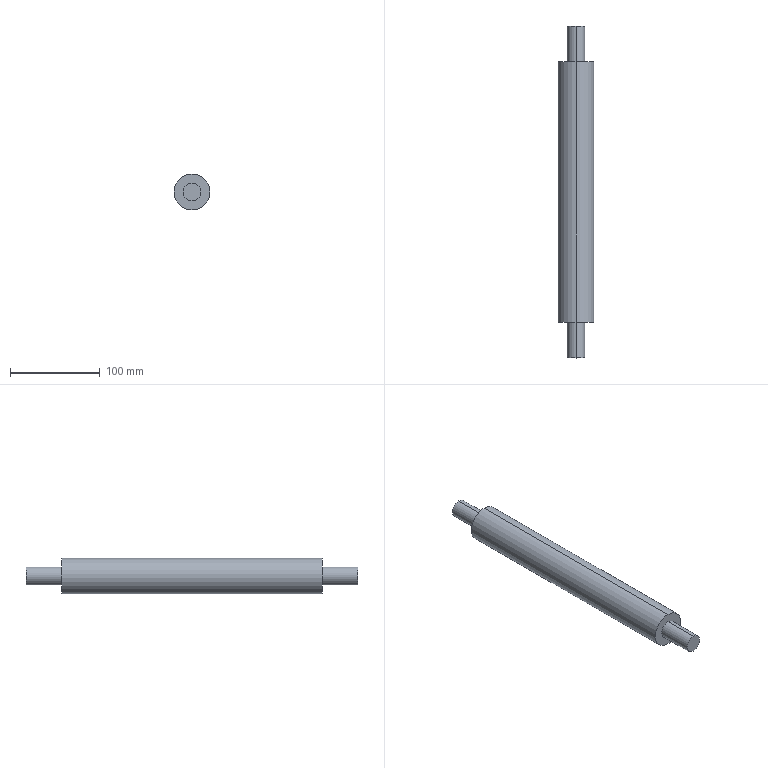Part | SolidWorks | features ICE 1, MirrorPattern 1, Revolution 1 | 1 solid | 20 faces | box 40 x 370 x 40 mm | volume 388983 mm3 | cylinder 10 | plane 10 | commonest cylinder face diameters 5 x4 20 x4 40 x2
STEP:
#1=CARTESIAN_POINT('',(0.,-145.,20.));
#2=VERTEX_POINT('',#1);
#3=CARTESIAN_POINT('',(0.,-145.,-20.));
#4=VERTEX_POINT('',#3);
#5=CARTESIAN_POINT('',(0.,-145.,0.));
#6=DIRECTION('',(0.,1.,0.));
#7=DIRECTION('',(0.,0.,1.));
#8=AXIS2_PLACEMENT_3D('',#5,#6,#7);
#9=CIRCLE('',#8,20.);
#10=EDGE_CURVE('',#2,#4,#9,.T.);
#11=ORIENTED_EDGE('',*,*,#10,.T.);
#12=CARTESIAN_POINT('',(0.,145.,-20.));
#13=VERTEX_POINT('',#12);
#14=CARTESIAN_POINT('',(0.,189.93,-20.));
#15=DIRECTION('',(0.,1.,0.));
#16=VECTOR('',#15,1000.);
#17=LINE('',#14,#16);
#18=EDGE_CURVE('',#4,#13,#17,.T.);
#19=ORIENTED_EDGE('',*,*,#18,.T.);
#20=CARTESIAN_POINT('',(0.,145.,20.));
#21=VERTEX_POINT('',#20);
#22=CARTESIAN_POINT('',(0.,145.,0.));
#23=DIRECTION('',(0.,1.,0.));
#24=DIRECTION('',(0.,0.,1.));
#25=AXIS2_PLACEMENT_3D('',#22,#23,#24);
#26=CIRCLE('',#25,20.);
#27=EDGE_CURVE('',#21,#13,#26,.T.);
#28=ORIENTED_EDGE('',*,*,#27,.F.);
#29=CARTESIAN_POINT('',(0.,189.93,20.));
#30=DIRECTION('',(0.,1.,0.));
#31=VECTOR('',#30,1000.);
#32=LINE('',#29,#31);
#33=EDGE_CURVE('',#2,#21,#32,.T.);
#34=ORIENTED_EDGE('',*,*,#33,.F.);
#35=EDGE_LOOP('',(#11,#19,#28,#34));
#36=FACE_OUTER_BOUND('',#35,.T.);
#37=CARTESIAN_POINT('',(0.,189.93,0.));
#38=DIRECTION('',(0.,1.,0.));
#39=DIRECTION('',(0.,0.,1.));
#40=AXIS2_PLACEMENT_3D('',#37,#38,#39);
#41=CYLINDRICAL_SURFACE('',#40,20.);
#42=ADVANCED_FACE('',(#36),#41,.T.);
#43=CARTESIAN_POINT('',(0.,145.,10.));
#44=VERTEX_POINT('',#43);
#45=CARTESIAN_POINT('',(0.,145.,-10.));
#46=VERTEX_POINT('',#45);
#47=CARTESIAN_POINT('',(0.,145.,0.));
#48=DIRECTION('',(0.,1.,0.));
#49=DIRECTION('',(0.,0.,1.));
#50=AXIS2_PLACEMENT_3D('',#47,#48,#49);
#51=CIRCLE('',#50,10.);
#52=EDGE_CURVE('',#44,#46,#51,.T.);
#53=ORIENTED_EDGE('',*,*,#52,.T.);
#54=CARTESIAN_POINT('',(0.,152.5,-10.));
#55=VERTEX_POINT('',#54);
#56=CARTESIAN_POINT('',(0.,189.93,-10.));
#57=DIRECTION('',(0.,1.,0.));
#58=VECTOR('',#57,1000.);
#59=LINE('',#56,#58);
#60=EDGE_CURVE('',#46,#55,#59,.T.);
#61=ORIENTED_EDGE('',*,*,#60,.T.);
#62=CARTESIAN_POINT('',(2.5,155.,-9.682));
#63=VERTEX_POINT('',#62);
#64=CARTESIAN_POINT('',(2.5,155.,-9.682));
#65=CARTESIAN_POINT('',(2.5,154.834,-9.682));
#66=CARTESIAN_POINT('',(2.484,154.671,-9.687));
#67=CARTESIAN_POINT('',(2.42,154.351,-9.703));
#68=CARTESIAN_POINT('',(2.371,154.191,-9.715));
#69=CARTESIAN_POINT('',(2.245,153.889,-9.745));
#70=CARTESIAN_POINT('',(2.169,153.745,-9.762));
#71=CARTESIAN_POINT('',(1.987,153.474,-9.801));
#72=CARTESIAN_POINT('',(1.882,153.346,-9.822));
#73=CARTESIAN_POINT('',(1.537,153.002,-9.884));
#74=CARTESIAN_POINT('',(1.259,152.816,-9.925));
#75=CARTESIAN_POINT('',(0.8081,152.629,-9.968));
#76=CARTESIAN_POINT('',(0.6497,152.58,-9.98));
#77=CARTESIAN_POINT('',(0.3266,152.516,-9.996));
#78=CARTESIAN_POINT('',(0.1638,152.5,-10.));
#79=CARTESIAN_POINT('',(0.,152.5,-10.));
#80=B_SPLINE_CURVE_WITH_KNOTS('',3,(#64,#65,#66,#67,#68,#69,#70,#71,#72,#73,#74,#75,#76,#77,#78,#79),.UNSPECIFIED.,.F.,.F.,(4,2,2,2,2,2,2,4),(0.,0.0004906,0.0009812,0.001472,0.001962,0.002944,0.003434,0.003925),.UNSPECIFIED.);
#81=EDGE_CURVE('',#63,#55,#80,.T.);
#82=ORIENTED_EDGE('',*,*,#81,.F.);
#83=CARTESIAN_POINT('',(2.5,175.,-9.682));
#84=VERTEX_POINT('',#83);
#85=CARTESIAN_POINT('',(2.5,189.93,-9.682));
#86=DIRECTION('',(0.,-1.,0.));
#87=VECTOR('',#86,1000.);
#88=LINE('',#85,#87);
#89=EDGE_CURVE('',#84,#63,#88,.T.);
#90=ORIENTED_EDGE('',*,*,#89,.F.);
#91=CARTESIAN_POINT('',(0.,177.5,-10.));
#92=VERTEX_POINT('',#91);
#93=CARTESIAN_POINT('',(0.,177.5,-10.));
#94=CARTESIAN_POINT('',(0.1637,177.5,-10.));
#95=CARTESIAN_POINT('',(0.3299,177.484,-9.996));
#96=CARTESIAN_POINT('',(0.6508,177.419,-9.98));
#97=CARTESIAN_POINT('',(0.8069,177.372,-9.969));
#98=CARTESIAN_POINT('',(1.262,177.183,-9.925));
#99=CARTESIAN_POINT('',(1.536,176.999,-9.884));
#100=CARTESIAN_POINT('',(1.884,176.652,-9.822));
#101=CARTESIAN_POINT('',(1.986,176.527,-9.801));
#102=CARTESIAN_POINT('',(2.167,176.257,-9.763));
#103=CARTESIAN_POINT('',(2.246,176.11,-9.745));
#104=CARTESIAN_POINT('',(2.371,175.809,-9.715));
#105=CARTESIAN_POINT('',(2.419,175.653,-9.703));
#106=CARTESIAN_POINT('',(2.483,175.332,-9.687));
#107=CARTESIAN_POINT('',(2.5,175.166,-9.682));
#108=CARTESIAN_POINT('',(2.5,175.,-9.682));
#109=B_SPLINE_CURVE_WITH_KNOTS('',3,(#93,#94,#95,#96,#97,#98,#99,#100,#101,#102,#103,#104,#105,#106,#107,#108),.UNSPECIFIED.,.F.,.F.,(4,2,2,2,2,2,2,4),(0.003925,0.004415,0.004905,0.005885,0.006375,0.006865,0.007355,0.007845),.UNSPECIFIED.);
#110=EDGE_CURVE('',#92,#84,#109,.T.);
#111=ORIENTED_EDGE('',*,*,#110,.F.);
#112=CARTESIAN_POINT('',(0.,185.,-10.));
#113=VERTEX_POINT('',#112);
#114=CARTESIAN_POINT('',(0.,189.93,-10.));
#115=DIRECTION('',(0.,1.,0.));
#116=VECTOR('',#115,1000.);
#117=LINE('',#114,#116);
#118=EDGE_CURVE('',#92,#113,#117,.T.);
#119=ORIENTED_EDGE('',*,*,#118,.T.);
#120=CARTESIAN_POINT('',(0.,185.,10.));
#121=VERTEX_POINT('',#120);
#122=CARTESIAN_POINT('',(0.,185.,0.));
#123=DIRECTION('',(0.,1.,0.));
#124=DIRECTION('',(0.,0.,1.));
#125=AXIS2_PLACEMENT_3D('',#122,#123,#124);
#126=CIRCLE('',#125,10.);
#127=EDGE_CURVE('',#121,#113,#126,.T.);
#128=ORIENTED_EDGE('',*,*,#127,.F.);
#129=CARTESIAN_POINT('',(0.,189.93,10.));
#130=DIRECTION('',(0.,1.,0.));
#131=VECTOR('',#130,1000.);
#132=LINE('',#129,#131);
#133=EDGE_CURVE('',#44,#121,#132,.T.);
#134=ORIENTED_EDGE('',*,*,#133,.F.);
#135=EDGE_LOOP('',(#53,#61,#82,#90,#111,#119,#128,#134));
#136=FACE_OUTER_BOUND('',#135,.T.);
#137=CARTESIAN_POINT('',(0.,189.93,0.));
#138=DIRECTION('',(0.,1.,0.));
#139=DIRECTION('',(0.,0.,1.));
#140=AXIS2_PLACEMENT_3D('',#137,#138,#139);
#141=CYLINDRICAL_SURFACE('',#140,10.);
#142=ADVANCED_FACE('',(#136),#141,.T.);
#143=CARTESIAN_POINT('',(0.,-185.,10.));
#144=VERTEX_POINT('',#143);
#145=CARTESIAN_POINT('',(0.,-185.,-10.));
#146=VERTEX_POINT('',#145);
#147=CARTESIAN_POINT('',(0.,-185.,0.));
#148=DIRECTION('',(0.,1.,0.));
#149=DIRECTION('',(0.,0.,1.));
#150=AXIS2_PLACEMENT_3D('',#147,#148,#149);
#151=CIRCLE('',#150,10.);
#152=EDGE_CURVE('',#144,#146,#151,.T.);
#153=ORIENTED_EDGE('',*,*,#152,.T.);
#154=CARTESIAN_POINT('',(0.,-177.5,-10.));
#155=VERTEX_POINT('',#154);
#156=CARTESIAN_POINT('',(0.,189.93,-10.));
#157=DIRECTION('',(0.,1.,0.));
#158=VECTOR('',#157,1000.);
#159=LINE('',#156,#158);
#160=EDGE_CURVE('',#146,#155,#159,.T.);
#161=ORIENTED_EDGE('',*,*,#160,.T.);
#162=CARTESIAN_POINT('',(2.5,-175.,-9.682));
#163=VERTEX_POINT('',#162);
#164=CARTESIAN_POINT('',(0.,-177.5,-10.));
#165=CARTESIAN_POINT('',(0.1637,-177.5,-10.));
#166=CARTESIAN_POINT('',(0.3299,-177.484,-9.996));
#167=CARTESIAN_POINT('',(0.6508,-177.419,-9.98));
#168=CARTESIAN_POINT('',(0.8069,-177.372,-9.969));
#169=CARTESIAN_POINT('',(1.262,-177.183,-9.925));
#170=CARTESIAN_POINT('',(1.536,-176.999,-9.884));
#171=CARTESIAN_POINT('',(1.884,-176.652,-9.822));
#172=CARTESIAN_POINT('',(1.986,-176.527,-9.801));
#173=CARTESIAN_POINT('',(2.167,-176.257,-9.763));
#174=CARTESIAN_POINT('',(2.246,-176.11,-9.745));
#175=CARTESIAN_POINT('',(2.371,-175.809,-9.715));
#176=CARTESIAN_POINT('',(2.419,-175.653,-9.703));
#177=CARTESIAN_POINT('',(2.483,-175.332,-9.687));
#178=CARTESIAN_POINT('',(2.5,-175.166,-9.682));
#179=CARTESIAN_POINT('',(2.5,-175.,-9.682));
#180=B_SPLINE_CURVE_WITH_KNOTS('',3,(#164,#165,#166,#167,#168,#169,#170,#171,#172,#173,#174,#175,#176,#177,#178,#179),.UNSPECIFIED.,.F.,.F.,(4,2,2,2,2,2,2,4),(0.003925,0.004415,0.004905,0.005885,0.006375,0.006865,0.007355,0.007845),.UNSPECIFIED.);
#181=EDGE_CURVE('',#155,#163,#180,.T.);
#182=ORIENTED_EDGE('',*,*,#181,.T.);
#183=CARTESIAN_POINT('',(2.5,-155.,-9.682));
#184=VERTEX_POINT('',#183);
#185=CARTESIAN_POINT('',(2.5,189.93,-9.682));
#186=DIRECTION('',(0.,1.,0.));
#187=VECTOR('',#186,1000.);
#188=LINE('',#185,#187);
#189=EDGE_CURVE('',#163,#184,#188,.T.);
#190=ORIENTED_EDGE('',*,*,#189,.T.);
#191=CARTESIAN_POINT('',(0.,-152.5,-10.));
#192=VERTEX_POINT('',#191);
#193=CARTESIAN_POINT('',(2.5,-155.,-9.682));
#194=CARTESIAN_POINT('',(2.5,-154.834,-9.682));
#195=CARTESIAN_POINT('',(2.484,-154.671,-9.687));
#196=CARTESIAN_POINT('',(2.42,-154.351,-9.703));
#197=CARTESIAN_POINT('',(2.371,-154.191,-9.715));
#198=CARTESIAN_POINT('',(2.245,-153.889,-9.745));
#199=CARTESIAN_POINT('',(2.169,-153.745,-9.762));
#200=CARTESIAN_POINT('',(1.987,-153.474,-9.801));
#201=CARTESIAN_POINT('',(1.882,-153.346,-9.822));
#202=CARTESIAN_POINT('',(1.537,-153.002,-9.884));
#203=CARTESIAN_POINT('',(1.259,-152.816,-9.925));
#204=CARTESIAN_POINT('',(0.8081,-152.629,-9.968));
#205=CARTESIAN_POINT('',(0.6497,-152.58,-9.98));
#206=CARTESIAN_POINT('',(0.3266,-152.516,-9.996));
#207=CARTESIAN_POINT('',(0.1638,-152.5,-10.));
#208=CARTESIAN_POINT('',(0.,-152.5,-10.));
#209=B_SPLINE_CURVE_WITH_KNOTS('',3,(#193,#194,#195,#196,#197,#198,#199,#200,#201,#202,#203,#204,#205,#206,#207,#208),.UNSPECIFIED.,.F.,.F.,(4,2,2,2,2,2,2,4),(0.,0.0004906,0.0009812,0.001472,0.001962,0.002944,0.003434,0.003925),.UNSPECIFIED.);
#210=EDGE_CURVE('',#184,#192,#209,.T.);
#211=ORIENTED_EDGE('',*,*,#210,.T.);
#212=CARTESIAN_POINT('',(0.,-145.,-10.));
#213=VERTEX_POINT('',#212);
#214=CARTESIAN_POINT('',(0.,189.93,-10.));
#215=DIRECTION('',(0.,1.,0.));
#216=VECTOR('',#215,1000.);
#217=LINE('',#214,#216);
#218=EDGE_CURVE('',#192,#213,#217,.T.);
#219=ORIENTED_EDGE('',*,*,#218,.T.);
#220=CARTESIAN_POINT('',(0.,-145.,10.));
#221=VERTEX_POINT('',#220);
#222=CARTESIAN_POINT('',(0.,-145.,0.));
#223=DIRECTION('',(0.,1.,0.));
#224=DIRECTION('',(0.,0.,1.));
#225=AXIS2_PLACEMENT_3D('',#222,#223,#224);
#226=CIRCLE('',#225,10.);
#227=EDGE_CURVE('',#221,#213,#226,.T.);
#228=ORIENTED_EDGE('',*,*,#227,.F.);
#229=CARTESIAN_POINT('',(0.,189.93,10.));
#230=DIRECTION('',(0.,1.,0.));
#231=VECTOR('',#230,1000.);
#232=LINE('',#229,#231);
#233=EDGE_CURVE('',#144,#221,#232,.T.);
#234=ORIENTED_EDGE('',*,*,#233,.F.);
#235=EDGE_LOOP('',(#153,#161,#182,#190,#211,#219,#228,#234));
#236=FACE_OUTER_BOUND('',#235,.T.);
#237=CARTESIAN_POINT('',(0.,189.93,0.));
#238=DIRECTION('',(0.,1.,0.));
#239=DIRECTION('',(0.,0.,1.));
#240=AXIS2_PLACEMENT_3D('',#237,#238,#239);
#241=CYLINDRICAL_SURFACE('',#240,10.);
#242=ADVANCED_FACE('',(#236),#241,.T.);
#243=ORIENTED_EDGE('',*,*,#160,.F.);
#244=CARTESIAN_POINT('',(0.,-185.,0.));
#245=DIRECTION('',(0.,1.,0.));
#246=DIRECTION('',(0.,0.,1.));
#247=AXIS2_PLACEMENT_3D('',#244,#245,#246);
#248=CIRCLE('',#247,10.);
#249=EDGE_CURVE('',#146,#144,#248,.T.);
#250=ORIENTED_EDGE('',*,*,#249,.T.);
#251=ORIENTED_EDGE('',*,*,#233,.T.);
#252=CARTESIAN_POINT('',(0.,-145.,0.));
#253=DIRECTION('',(0.,1.,0.));
#254=DIRECTION('',(0.,0.,1.));
#255=AXIS2_PLACEMENT_3D('',#252,#253,#254);
#256=CIRCLE('',#255,10.);
#257=EDGE_CURVE('',#213,#221,#256,.T.);
#258=ORIENTED_EDGE('',*,*,#257,.F.);
#259=ORIENTED_EDGE('',*,*,#218,.F.);
#260=CARTESIAN_POINT('',(-2.5,-155.,-9.682));
#261=VERTEX_POINT('',#260);
#262=CARTESIAN_POINT('',(0.,-152.5,-10.));
#263=CARTESIAN_POINT('',(-0.1637,-152.5,-10.));
#264=CARTESIAN_POINT('',(-0.3299,-152.516,-9.996));
#265=CARTESIAN_POINT('',(-0.6508,-152.581,-9.98));
#266=CARTESIAN_POINT('',(-0.8069,-152.628,-9.969));
#267=CARTESIAN_POINT('',(-1.262,-152.817,-9.925));
#268=CARTESIAN_POINT('',(-1.536,-153.001,-9.884));
#269=CARTESIAN_POINT('',(-1.884,-153.348,-9.822));
#270=CARTESIAN_POINT('',(-1.986,-153.473,-9.801));
#271=CARTESIAN_POINT('',(-2.167,-153.743,-9.763));
#272=CARTESIAN_POINT('',(-2.246,-153.89,-9.745));
#273=CARTESIAN_POINT('',(-2.371,-154.191,-9.715));
#274=CARTESIAN_POINT('',(-2.419,-154.347,-9.703));
#275=CARTESIAN_POINT('',(-2.483,-154.668,-9.687));
#276=CARTESIAN_POINT('',(-2.5,-154.834,-9.682));
#277=CARTESIAN_POINT('',(-2.5,-155.,-9.682));
#278=B_SPLINE_CURVE_WITH_KNOTS('',3,(#262,#263,#264,#265,#266,#267,#268,#269,#270,#271,#272,#273,#274,#275,#276,#277),.UNSPECIFIED.,.F.,.F.,(4,2,2,2,2,2,2,4),(0.003925,0.004415,0.004905,0.005885,0.006375,0.006865,0.007355,0.007845),.UNSPECIFIED.);
#279=EDGE_CURVE('',#192,#261,#278,.T.);
#280=ORIENTED_EDGE('',*,*,#279,.T.);
#281=CARTESIAN_POINT('',(-2.5,-175.,-9.682));
#282=VERTEX_POINT('',#281);
#283=CARTESIAN_POINT('',(-2.5,189.93,-9.682));
#284=DIRECTION('',(0.,-1.,0.));
#285=VECTOR('',#284,1000.);
#286=LINE('',#283,#285);
#287=EDGE_CURVE('',#261,#282,#286,.T.);
#288=ORIENTED_EDGE('',*,*,#287,.T.);
#289=CARTESIAN_POINT('',(-2.5,-175.,-9.682));
#290=CARTESIAN_POINT('',(-2.5,-175.166,-9.682));
#291=CARTESIAN_POINT('',(-2.484,-175.329,-9.687));
#292=CARTESIAN_POINT('',(-2.42,-175.649,-9.703));
#293=CARTESIAN_POINT('',(-2.371,-175.809,-9.715));
#294=CARTESIAN_POINT('',(-2.245,-176.111,-9.745));
#295=CARTESIAN_POINT('',(-2.169,-176.255,-9.762));
#296=CARTESIAN_POINT('',(-1.987,-176.526,-9.801));
#297=CARTESIAN_POINT('',(-1.882,-176.654,-9.822));
#298=CARTESIAN_POINT('',(-1.537,-176.998,-9.884));
#299=CARTESIAN_POINT('',(-1.259,-177.184,-9.925));
#300=CARTESIAN_POINT('',(-0.8081,-177.371,-9.968));
#301=CARTESIAN_POINT('',(-0.6497,-177.42,-9.98));
#302=CARTESIAN_POINT('',(-0.3266,-177.484,-9.996));
#303=CARTESIAN_POINT('',(-0.1638,-177.5,-10.));
#304=CARTESIAN_POINT('',(0.,-177.5,-10.));
#305=B_SPLINE_CURVE_WITH_KNOTS('',3,(#289,#290,#291,#292,#293,#294,#295,#296,#297,#298,#299,#300,#301,#302,#303,#304),.UNSPECIFIED.,.F.,.F.,(4,2,2,2,2,2,2,4),(0.,0.0004906,0.0009812,0.001472,0.001962,0.002944,0.003434,0.003925),.UNSPECIFIED.);
#306=EDGE_CURVE('',#282,#155,#305,.T.);
#307=ORIENTED_EDGE('',*,*,#306,.T.);
#308=EDGE_LOOP('',(#243,#250,#251,#258,#259,#280,#288,#307));
#309=FACE_OUTER_BOUND('',#308,.T.);
#310=CARTESIAN_POINT('',(0.,189.93,0.));
#311=DIRECTION('',(0.,1.,0.));
#312=DIRECTION('',(0.,0.,1.));
#313=AXIS2_PLACEMENT_3D('',#310,#311,#312);
#314=CYLINDRICAL_SURFACE('',#313,10.);
#315=ADVANCED_FACE('',(#309),#314,.T.);
#316=ORIENTED_EDGE('',*,*,#127,.T.);
#317=CARTESIAN_POINT('',(0.,185.,0.));
#318=DIRECTION('',(0.,1.,0.));
#319=DIRECTION('',(0.,0.,1.));
#320=AXIS2_PLACEMENT_3D('',#317,#318,#319);
#321=CIRCLE('',#320,10.);
#322=EDGE_CURVE('',#113,#121,#321,.T.);
#323=ORIENTED_EDGE('',*,*,#322,.T.);
#324=EDGE_LOOP('',(#316,#323));
#325=FACE_OUTER_BOUND('',#324,.T.);
#326=CARTESIAN_POINT('',(0.,185.,0.));
#327=DIRECTION('',(0.,1.,0.));
#328=DIRECTION('',(0.,0.,1.));
#329=AXIS2_PLACEMENT_3D('',#326,#327,#328);
#330=PLANE('',#329);
#331=ADVANCED_FACE('',(#325),#330,.T.);
#332=ORIENTED_EDGE('',*,*,#60,.F.);
#333=CARTESIAN_POINT('',(0.,145.,0.));
#334=DIRECTION('',(0.,1.,0.));
#335=DIRECTION('',(0.,0.,1.));
#336=AXIS2_PLACEMENT_3D('',#333,#334,#335);
#337=CIRCLE('',#336,10.);
#338=EDGE_CURVE('',#46,#44,#337,.T.);
#339=ORIENTED_EDGE('',*,*,#338,.T.);
#340=ORIENTED_EDGE('',*,*,#133,.T.);
#341=ORIENTED_EDGE('',*,*,#322,.F.);
#342=ORIENTED_EDGE('',*,*,#118,.F.);
#343=CARTESIAN_POINT('',(-2.5,175.,-9.682));
#344=VERTEX_POINT('',#343);
#345=CARTESIAN_POINT('',(-2.5,175.,-9.682));
#346=CARTESIAN_POINT('',(-2.5,175.166,-9.682));
#347=CARTESIAN_POINT('',(-2.484,175.329,-9.687));
#348=CARTESIAN_POINT('',(-2.42,175.649,-9.703));
#349=CARTESIAN_POINT('',(-2.371,175.809,-9.715));
#350=CARTESIAN_POINT('',(-2.245,176.111,-9.745));
#351=CARTESIAN_POINT('',(-2.169,176.255,-9.762));
#352=CARTESIAN_POINT('',(-1.987,176.526,-9.801));
#353=CARTESIAN_POINT('',(-1.882,176.654,-9.822));
#354=CARTESIAN_POINT('',(-1.537,176.998,-9.884));
#355=CARTESIAN_POINT('',(-1.259,177.184,-9.925));
#356=CARTESIAN_POINT('',(-0.8081,177.371,-9.968));
#357=CARTESIAN_POINT('',(-0.6497,177.42,-9.98));
#358=CARTESIAN_POINT('',(-0.3266,177.484,-9.996));
#359=CARTESIAN_POINT('',(-0.1638,177.5,-10.));
#360=CARTESIAN_POINT('',(0.,177.5,-10.));
#361=B_SPLINE_CURVE_WITH_KNOTS('',3,(#345,#346,#347,#348,#349,#350,#351,#352,#353,#354,#355,#356,#357,#358,#359,#360),.UNSPECIFIED.,.F.,.F.,(4,2,2,2,2,2,2,4),(0.,0.0004906,0.0009812,0.001472,0.001962,0.002944,0.003434,0.003925),.UNSPECIFIED.);
#362=EDGE_CURVE('',#344,#92,#361,.T.);
#363=ORIENTED_EDGE('',*,*,#362,.F.);
#364=CARTESIAN_POINT('',(-2.5,155.,-9.682));
#365=VERTEX_POINT('',#364);
#366=CARTESIAN_POINT('',(-2.5,189.93,-9.682));
#367=DIRECTION('',(0.,1.,0.));
#368=VECTOR('',#367,1000.);
#369=LINE('',#366,#368);
#370=EDGE_CURVE('',#365,#344,#369,.T.);
#371=ORIENTED_EDGE('',*,*,#370,.F.);
#372=CARTESIAN_POINT('',(0.,152.5,-10.));
#373=CARTESIAN_POINT('',(-0.1637,152.5,-10.));
#374=CARTESIAN_POINT('',(-0.3299,152.516,-9.996));
#375=CARTESIAN_POINT('',(-0.6508,152.581,-9.98));
#376=CARTESIAN_POINT('',(-0.8069,152.628,-9.969));
#377=CARTESIAN_POINT('',(-1.262,152.817,-9.925));
#378=CARTESIAN_POINT('',(-1.536,153.001,-9.884));
#379=CARTESIAN_POINT('',(-1.884,153.348,-9.822));
#380=CARTESIAN_POINT('',(-1.986,153.473,-9.801));
#381=CARTESIAN_POINT('',(-2.167,153.743,-9.763));
#382=CARTESIAN_POINT('',(-2.246,153.89,-9.745));
#383=CARTESIAN_POINT('',(-2.371,154.191,-9.715));
#384=CARTESIAN_POINT('',(-2.419,154.347,-9.703));
#385=CARTESIAN_POINT('',(-2.483,154.668,-9.687));
#386=CARTESIAN_POINT('',(-2.5,154.834,-9.682));
#387=CARTESIAN_POINT('',(-2.5,155.,-9.682));
#388=B_SPLINE_CURVE_WITH_KNOTS('',3,(#372,#373,#374,#375,#376,#377,#378,#379,#380,#381,#382,#383,#384,#385,#386,#387),.UNSPECIFIED.,.F.,.F.,(4,2,2,2,2,2,2,4),(0.003925,0.004415,0.004905,0.005885,0.006375,0.006865,0.007355,0.007845),.UNSPECIFIED.);
#389=EDGE_CURVE('',#55,#365,#388,.T.);
#390=ORIENTED_EDGE('',*,*,#389,.F.);
#391=EDGE_LOOP('',(#332,#339,#340,#341,#342,#363,#371,#390));
#392=FACE_OUTER_BOUND('',#391,.T.);
#393=CARTESIAN_POINT('',(0.,189.93,0.));
#394=DIRECTION('',(0.,1.,0.));
#395=DIRECTION('',(0.,0.,1.));
#396=AXIS2_PLACEMENT_3D('',#393,#394,#395);
#397=CYLINDRICAL_SURFACE('',#396,10.);
#398=ADVANCED_FACE('',(#392),#397,.T.);
#399=ORIENTED_EDGE('',*,*,#27,.T.);
#400=CARTESIAN_POINT('',(0.,145.,0.));
#401=DIRECTION('',(0.,1.,0.));
#402=DIRECTION('',(0.,0.,1.));
#403=AXIS2_PLACEMENT_3D('',#400,#401,#402);
#404=CIRCLE('',#403,20.);
#405=EDGE_CURVE('',#13,#21,#404,.T.);
#406=ORIENTED_EDGE('',*,*,#405,.T.);
#407=EDGE_LOOP('',(#399,#406));
#408=FACE_OUTER_BOUND('',#407,.T.);
#409=ORIENTED_EDGE('',*,*,#52,.F.);
#410=ORIENTED_EDGE('',*,*,#338,.F.);
#411=EDGE_LOOP('',(#409,#410));
#412=FACE_BOUND('',#411,.T.);
#413=CARTESIAN_POINT('',(0.,145.,10.));
#414=DIRECTION('',(0.,1.,0.));
#415=DIRECTION('',(0.,0.,1.));
#416=AXIS2_PLACEMENT_3D('',#413,#414,#415);
#417=PLANE('',#416);
#418=ADVANCED_FACE('',(#408,#412),#417,.T.);
#419=ORIENTED_EDGE('',*,*,#18,.F.);
#420=CARTESIAN_POINT('',(0.,-145.,0.));
#421=DIRECTION('',(0.,1.,0.));
#422=DIRECTION('',(0.,0.,1.));
#423=AXIS2_PLACEMENT_3D('',#420,#421,#422);
#424=CIRCLE('',#423,20.);
#425=EDGE_CURVE('',#4,#2,#424,.T.);
#426=ORIENTED_EDGE('',*,*,#425,.T.);
#427=ORIENTED_EDGE('',*,*,#33,.T.);
#428=ORIENTED_EDGE('',*,*,#405,.F.);
#429=EDGE_LOOP('',(#419,#426,#427,#428));
#430=FACE_OUTER_BOUND('',#429,.T.);
#431=CARTESIAN_POINT('',(0.,189.93,0.));
#432=DIRECTION('',(0.,1.,0.));
#433=DIRECTION('',(0.,0.,1.));
#434=AXIS2_PLACEMENT_3D('',#431,#432,#433);
#435=CYLINDRICAL_SURFACE('',#434,20.);
#436=ADVANCED_FACE('',(#430),#435,.T.);
#437=ORIENTED_EDGE('',*,*,#227,.T.);
#438=ORIENTED_EDGE('',*,*,#257,.T.);
#439=EDGE_LOOP('',(#437,#438));
#440=FACE_BOUND('',#439,.T.);
#441=ORIENTED_EDGE('',*,*,#10,.F.);
#442=ORIENTED_EDGE('',*,*,#425,.F.);
#443=EDGE_LOOP('',(#441,#442));
#444=FACE_OUTER_BOUND('',#443,.T.);
#445=CARTESIAN_POINT('',(0.,-145.,20.));
#446=DIRECTION('',(0.,-1.,0.));
#447=DIRECTION('',(0.,0.,-1.));
#448=AXIS2_PLACEMENT_3D('',#445,#446,#447);
#449=PLANE('',#448);
#450=ADVANCED_FACE('',(#440,#444),#449,.T.);
#451=ORIENTED_EDGE('',*,*,#152,.F.);
#452=ORIENTED_EDGE('',*,*,#249,.F.);
#453=EDGE_LOOP('',(#451,#452));
#454=FACE_OUTER_BOUND('',#453,.T.);
#455=CARTESIAN_POINT('',(0.,-185.,10.));
#456=DIRECTION('',(0.,-1.,0.));
#457=DIRECTION('',(0.,0.,-1.));
#458=AXIS2_PLACEMENT_3D('',#455,#456,#457);
#459=PLANE('',#458);
#460=ADVANCED_FACE('',(#454),#459,.T.);
#461=CARTESIAN_POINT('',(-2.5,175.,-7.5));
#462=VERTEX_POINT('',#461);
#463=CARTESIAN_POINT('',(-2.5,175.,-7.5));
#464=DIRECTION('',(0.,0.,-1.));
#465=VECTOR('',#464,1000.);
#466=LINE('',#463,#465);
#467=EDGE_CURVE('',#462,#344,#466,.T.);
#468=ORIENTED_EDGE('',*,*,#467,.T.);
#469=ORIENTED_EDGE('',*,*,#362,.T.);
#470=ORIENTED_EDGE('',*,*,#110,.T.);
#471=CARTESIAN_POINT('',(2.5,175.,-7.5));
#472=VERTEX_POINT('',#471);
#473=CARTESIAN_POINT('',(2.5,175.,-7.5));
#474=DIRECTION('',(0.,0.,-1.));
#475=VECTOR('',#474,1000.);
#476=LINE('',#473,#475);
#477=EDGE_CURVE('',#472,#84,#476,.T.);
#478=ORIENTED_EDGE('',*,*,#477,.F.);
#479=CARTESIAN_POINT('',(0.,175.,-7.5));
#480=DIRECTION('',(0.,0.,-1.));
#481=DIRECTION('',(-1.,0.,0.));
#482=AXIS2_PLACEMENT_3D('',#479,#480,#481);
#483=CIRCLE('',#482,2.5);
#484=EDGE_CURVE('',#462,#472,#483,.T.);
#485=ORIENTED_EDGE('',*,*,#484,.F.);
#486=EDGE_LOOP('',(#468,#469,#470,#478,#485));
#487=FACE_OUTER_BOUND('',#486,.T.);
#488=CARTESIAN_POINT('',(0.,175.,-7.5));
#489=DIRECTION('',(0.,0.,-1.));
#490=DIRECTION('',(-1.,0.,0.));
#491=AXIS2_PLACEMENT_3D('',#488,#489,#490);
#492=CYLINDRICAL_SURFACE('',#491,2.5);
#493=ADVANCED_FACE('',(#487),#492,.F.);
#494=ORIENTED_EDGE('',*,*,#370,.T.);
#495=ORIENTED_EDGE('',*,*,#467,.F.);
#496=CARTESIAN_POINT('',(-2.5,155.,-7.5));
#497=VERTEX_POINT('',#496);
#498=CARTESIAN_POINT('',(-2.5,175.,-7.5));
#499=DIRECTION('',(0.,1.,0.));
#500=VECTOR('',#499,1000.);
#501=LINE('',#498,#500);
#502=EDGE_CURVE('',#497,#462,#501,.T.);
#503=ORIENTED_EDGE('',*,*,#502,.F.);
#504=CARTESIAN_POINT('',(-2.5,155.,-7.5));
#505=DIRECTION('',(0.,0.,-1.));
#506=VECTOR('',#505,1000.);
#507=LINE('',#504,#506);
#508=EDGE_CURVE('',#497,#365,#507,.T.);
#509=ORIENTED_EDGE('',*,*,#508,.T.);
#510=EDGE_LOOP('',(#494,#495,#503,#509));
#511=FACE_OUTER_BOUND('',#510,.T.);
#512=CARTESIAN_POINT('',(-2.5,175.,-7.5));
#513=DIRECTION('',(-1.,0.,0.));
#514=DIRECTION('',(0.,-1.,0.));
#515=AXIS2_PLACEMENT_3D('',#512,#513,#514);
#516=PLANE('',#515);
#517=ADVANCED_FACE('',(#511),#516,.F.);
#518=CARTESIAN_POINT('',(2.5,155.,-7.5));
#519=VERTEX_POINT('',#518);
#520=CARTESIAN_POINT('',(2.5,155.,-7.5));
#521=DIRECTION('',(0.,0.,-1.));
#522=VECTOR('',#521,1000.);
#523=LINE('',#520,#522);
#524=EDGE_CURVE('',#519,#63,#523,.T.);
#525=ORIENTED_EDGE('',*,*,#524,.T.);
#526=ORIENTED_EDGE('',*,*,#81,.T.);
#527=ORIENTED_EDGE('',*,*,#389,.T.);
#528=ORIENTED_EDGE('',*,*,#508,.F.);
#529=CARTESIAN_POINT('',(0.,155.,-7.5));
#530=DIRECTION('',(0.,0.,-1.));
#531=DIRECTION('',(-1.,0.,0.));
#532=AXIS2_PLACEMENT_3D('',#529,#530,#531);
#533=CIRCLE('',#532,2.5);
#534=EDGE_CURVE('',#519,#497,#533,.T.);
#535=ORIENTED_EDGE('',*,*,#534,.F.);
#536=EDGE_LOOP('',(#525,#526,#527,#528,#535));
#537=FACE_OUTER_BOUND('',#536,.T.);
#538=CARTESIAN_POINT('',(0.,155.,-7.5));
#539=DIRECTION('',(0.,0.,-1.));
#540=DIRECTION('',(-1.,0.,0.));
#541=AXIS2_PLACEMENT_3D('',#538,#539,#540);
#542=CYLINDRICAL_SURFACE('',#541,2.5);
#543=ADVANCED_FACE('',(#537),#542,.F.);
#544=ORIENTED_EDGE('',*,*,#89,.T.);
#545=ORIENTED_EDGE('',*,*,#524,.F.);
#546=CARTESIAN_POINT('',(2.5,175.,-7.5));
#547=DIRECTION('',(0.,-1.,0.));
#548=VECTOR('',#547,1000.);
#549=LINE('',#546,#548);
#550=EDGE_CURVE('',#472,#519,#549,.T.);
#551=ORIENTED_EDGE('',*,*,#550,.F.);
#552=ORIENTED_EDGE('',*,*,#477,.T.);
#553=EDGE_LOOP('',(#544,#545,#551,#552));
#554=FACE_OUTER_BOUND('',#553,.T.);
#555=CARTESIAN_POINT('',(2.5,175.,-7.5));
#556=DIRECTION('',(1.,0.,0.));
#557=DIRECTION('',(0.,1.,0.));
#558=AXIS2_PLACEMENT_3D('',#555,#556,#557);
#559=PLANE('',#558);
#560=ADVANCED_FACE('',(#554),#559,.F.);
#561=ORIENTED_EDGE('',*,*,#484,.T.);
#562=ORIENTED_EDGE('',*,*,#550,.T.);
#563=ORIENTED_EDGE('',*,*,#534,.T.);
#564=ORIENTED_EDGE('',*,*,#502,.T.);
#565=EDGE_LOOP('',(#561,#562,#563,#564));
#566=FACE_OUTER_BOUND('',#565,.T.);
#567=CARTESIAN_POINT('',(0.,175.,-7.5));
#568=DIRECTION('',(0.,0.,-1.));
#569=DIRECTION('',(-1.,0.,0.));
#570=AXIS2_PLACEMENT_3D('',#567,#568,#569);
#571=PLANE('',#570);
#572=ADVANCED_FACE('',(#566),#571,.T.);
#573=CARTESIAN_POINT('',(-2.5,-175.,-7.5));
#574=VERTEX_POINT('',#573);
#575=CARTESIAN_POINT('',(-2.5,-175.,-7.5));
#576=DIRECTION('',(0.,0.,-1.));
#577=VECTOR('',#576,1000.);
#578=LINE('',#575,#577);
#579=EDGE_CURVE('',#574,#282,#578,.T.);
#580=ORIENTED_EDGE('',*,*,#579,.F.);
#581=CARTESIAN_POINT('',(2.5,-175.,-7.5));
#582=VERTEX_POINT('',#581);
#583=CARTESIAN_POINT('',(0.,-175.,-7.5));
#584=DIRECTION('',(0.,0.,1.));
#585=DIRECTION('',(-1.,0.,0.));
#586=AXIS2_PLACEMENT_3D('',#583,#584,#585);
#587=CIRCLE('',#586,2.5);
#588=EDGE_CURVE('',#574,#582,#587,.T.);
#589=ORIENTED_EDGE('',*,*,#588,.T.);
#590=CARTESIAN_POINT('',(2.5,-175.,-7.5));
#591=DIRECTION('',(0.,0.,-1.));
#592=VECTOR('',#591,1000.);
#593=LINE('',#590,#592);
#594=EDGE_CURVE('',#582,#163,#593,.T.);
#595=ORIENTED_EDGE('',*,*,#594,.T.);
#596=ORIENTED_EDGE('',*,*,#181,.F.);
#597=ORIENTED_EDGE('',*,*,#306,.F.);
#598=EDGE_LOOP('',(#580,#589,#595,#596,#597));
#599=FACE_OUTER_BOUND('',#598,.T.);
#600=CARTESIAN_POINT('',(0.,-175.,-7.5));
#601=DIRECTION('',(0.,0.,-1.));
#602=DIRECTION('',(-1.,0.,0.));
#603=AXIS2_PLACEMENT_3D('',#600,#601,#602);
#604=CYLINDRICAL_SURFACE('',#603,2.5);
#605=ADVANCED_FACE('',(#599),#604,.F.);
#606=ORIENTED_EDGE('',*,*,#594,.F.);
#607=CARTESIAN_POINT('',(2.5,-155.,-7.5));
#608=VERTEX_POINT('',#607);
#609=CARTESIAN_POINT('',(2.5,-175.,-7.5));
#610=DIRECTION('',(0.,1.,0.));
#611=VECTOR('',#610,1000.);
#612=LINE('',#609,#611);
#613=EDGE_CURVE('',#582,#608,#612,.T.);
#614=ORIENTED_EDGE('',*,*,#613,.T.);
#615=CARTESIAN_POINT('',(2.5,-155.,-7.5));
#616=DIRECTION('',(0.,0.,-1.));
#617=VECTOR('',#616,1000.);
#618=LINE('',#615,#617);
#619=EDGE_CURVE('',#608,#184,#618,.T.);
#620=ORIENTED_EDGE('',*,*,#619,.T.);
#621=ORIENTED_EDGE('',*,*,#189,.F.);
#622=EDGE_LOOP('',(#606,#614,#620,#621));
#623=FACE_OUTER_BOUND('',#622,.T.);
#624=CARTESIAN_POINT('',(2.5,-175.,-7.5));
#625=DIRECTION('',(-1.,0.,0.));
#626=DIRECTION('',(0.,-1.,0.));
#627=AXIS2_PLACEMENT_3D('',#624,#625,#626);
#628=PLANE('',#627);
#629=ADVANCED_FACE('',(#623),#628,.T.);
#630=ORIENTED_EDGE('',*,*,#619,.F.);
#631=CARTESIAN_POINT('',(-2.5,-155.,-7.5));
#632=VERTEX_POINT('',#631);
#633=CARTESIAN_POINT('',(0.,-155.,-7.5));
#634=DIRECTION('',(0.,0.,1.));
#635=DIRECTION('',(-1.,0.,0.));
#636=AXIS2_PLACEMENT_3D('',#633,#634,#635);
#637=CIRCLE('',#636,2.5);
#638=EDGE_CURVE('',#608,#632,#637,.T.);
#639=ORIENTED_EDGE('',*,*,#638,.T.);
#640=CARTESIAN_POINT('',(-2.5,-155.,-7.5));
#641=DIRECTION('',(0.,0.,-1.));
#642=VECTOR('',#641,1000.);
#643=LINE('',#640,#642);
#644=EDGE_CURVE('',#632,#261,#643,.T.);
#645=ORIENTED_EDGE('',*,*,#644,.T.);
#646=ORIENTED_EDGE('',*,*,#279,.F.);
#647=ORIENTED_EDGE('',*,*,#210,.F.);
#648=EDGE_LOOP('',(#630,#639,#645,#646,#647));
#649=FACE_OUTER_BOUND('',#648,.T.);
#650=CARTESIAN_POINT('',(0.,-155.,-7.5));
#651=DIRECTION('',(0.,0.,-1.));
#652=DIRECTION('',(-1.,0.,0.));
#653=AXIS2_PLACEMENT_3D('',#650,#651,#652);
#654=CYLINDRICAL_SURFACE('',#653,2.5);
#655=ADVANCED_FACE('',(#649),#654,.F.);
#656=ORIENTED_EDGE('',*,*,#644,.F.);
#657=CARTESIAN_POINT('',(-2.5,-175.,-7.5));
#658=DIRECTION('',(0.,-1.,0.));
#659=VECTOR('',#658,1000.);
#660=LINE('',#657,#659);
#661=EDGE_CURVE('',#632,#574,#660,.T.);
#662=ORIENTED_EDGE('',*,*,#661,.T.);
#663=ORIENTED_EDGE('',*,*,#579,.T.);
#664=ORIENTED_EDGE('',*,*,#287,.F.);
#665=EDGE_LOOP('',(#656,#662,#663,#664));
#666=FACE_OUTER_BOUND('',#665,.T.);
#667=CARTESIAN_POINT('',(-2.5,-175.,-7.5));
#668=DIRECTION('',(1.,0.,0.));
#669=DIRECTION('',(0.,1.,0.));
#670=AXIS2_PLACEMENT_3D('',#667,#668,#669);
#671=PLANE('',#670);
#672=ADVANCED_FACE('',(#666),#671,.T.);
#673=ORIENTED_EDGE('',*,*,#588,.F.);
#674=ORIENTED_EDGE('',*,*,#661,.F.);
#675=ORIENTED_EDGE('',*,*,#638,.F.);
#676=ORIENTED_EDGE('',*,*,#613,.F.);
#677=EDGE_LOOP('',(#673,#674,#675,#676));
#678=FACE_OUTER_BOUND('',#677,.T.);
#679=CARTESIAN_POINT('',(0.,-175.,-7.5));
#680=DIRECTION('',(0.,0.,-1.));
#681=DIRECTION('',(-1.,0.,0.));
#682=AXIS2_PLACEMENT_3D('',#679,#680,#681);
#683=PLANE('',#682);
#684=ADVANCED_FACE('',(#678),#683,.T.);
#685=CLOSED_SHELL('',(#42,#142,#242,#315,#331,#398,#418,#436,#450,#460,#493,#517,#543,#560,#572,#605,#629,#655,#672,#684));
#686=MANIFOLD_SOLID_BREP('',#685);
#687=CARTESIAN_POINT('',(0.,0.,0.));
#688=DIRECTION('',(0.,0.,1.));
#689=DIRECTION('',(1.,0.,0.));
#690=AXIS2_PLACEMENT_3D('',#687,#688,#689);
#691=(LENGTH_UNIT()NAMED_UNIT(*)SI_UNIT(.MILLI.,.METRE.));
#692=UNCERTAINTY_MEASURE_WITH_UNIT(LENGTH_MEASURE(0.00001),#691,'','');
#693=(NAMED_UNIT(*)PLANE_ANGLE_UNIT()SI_UNIT($,.RADIAN.));
#694=(NAMED_UNIT(*)SI_UNIT($,.STERADIAN.)SOLID_ANGLE_UNIT());
#695=(GEOMETRIC_REPRESENTATION_CONTEXT(3)GLOBAL_UNCERTAINTY_ASSIGNED_CONTEXT((#692))GLOBAL_UNIT_ASSIGNED_CONTEXT((#691,#693,#694))REPRESENTATION_CONTEXT('',''));
#696=ADVANCED_BREP_SHAPE_REPRESENTATION('',(#686,#690),#695);